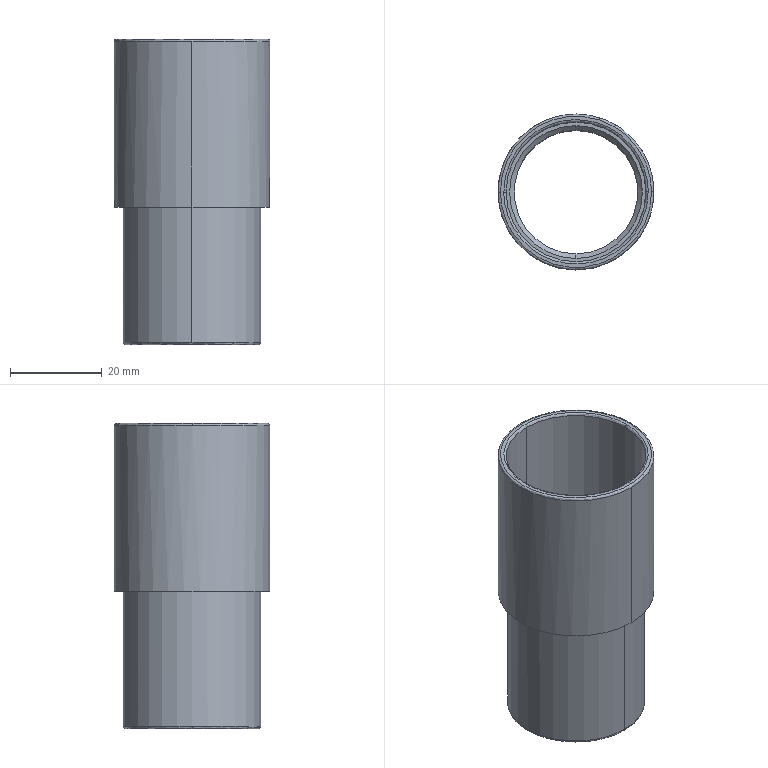Part | SolidWorks | features BaseBody 1 | 1 solid | 20 faces | box 34 x 34 x 66.6 mm | volume 12274 mm3 | cylinder 8 | spline 6 | plane 4 | cone 2 | commonest cylinder face diameters 27 x2 30 x2 30.5 x2 34 x2
STEP:
#1=CARTESIAN_POINT('',(464.037,37.643,-16.634));
#2=VERTEX_POINT('',#1);
#3=CARTESIAN_POINT('',(497.037,37.787,-16.634));
#4=VERTEX_POINT('',#3);
#5=CARTESIAN_POINT('',(464.037,37.643,-16.634));
#6=CARTESIAN_POINT('',(463.893,70.643,-16.634));
#7=CARTESIAN_POINT('',(496.893,70.786,-16.634));
#8=CARTESIAN_POINT('',(497.037,37.787,-16.634));
#9=(BOUNDED_CURVE()B_SPLINE_CURVE(3,(#5,#6,#7,#8),.UNSPECIFIED.,.F.,.T.)B_SPLINE_CURVE_WITH_KNOTS((4,4),(0.,1.),.UNSPECIFIED.)CURVE()GEOMETRIC_REPRESENTATION_ITEM()RATIONAL_B_SPLINE_CURVE((1.,0.3333,0.3333,1.))REPRESENTATION_ITEM(''));
#10=EDGE_CURVE('',#2,#4,#9,.T.);
#11=ORIENTED_EDGE('',*,*,#10,.T.);
#12=CARTESIAN_POINT('',(497.537,37.789,-17.134));
#13=VERTEX_POINT('',#12);
#14=CARTESIAN_POINT('',(497.037,37.787,-17.134));
#15=DIRECTION('',(-0.004352,1.,0.000000003));
#16=DIRECTION('',(1.,0.004352,-0.000000001));
#17=AXIS2_PLACEMENT_3D('',#14,#15,#16);
#18=CIRCLE('',#17,0.5);
#19=EDGE_CURVE('',#4,#13,#18,.T.);
#20=ORIENTED_EDGE('',*,*,#19,.T.);
#21=CARTESIAN_POINT('',(480.537,54.715,-17.134));
#22=VERTEX_POINT('',#21);
#23=CARTESIAN_POINT('',(480.537,37.715,-17.134));
#24=DIRECTION('',(-0.000000001,0.000000003,-1.));
#25=DIRECTION('',(0.,1.,0.000000003));
#26=AXIS2_PLACEMENT_3D('',#23,#24,#25);
#27=CIRCLE('',#26,17.);
#28=EDGE_CURVE('',#22,#13,#27,.T.);
#29=ORIENTED_EDGE('',*,*,#28,.F.);
#30=CARTESIAN_POINT('',(463.537,37.641,-17.134));
#31=VERTEX_POINT('',#30);
#32=CARTESIAN_POINT('',(480.537,37.715,-17.134));
#33=DIRECTION('',(-0.000000001,0.000000003,-1.));
#34=DIRECTION('',(0.,1.,0.000000003));
#35=AXIS2_PLACEMENT_3D('',#32,#33,#34);
#36=CIRCLE('',#35,17.);
#37=EDGE_CURVE('',#31,#22,#36,.T.);
#38=ORIENTED_EDGE('',*,*,#37,.F.);
#39=CARTESIAN_POINT('',(464.037,37.643,-17.134));
#40=DIRECTION('',(0.004352,-1.,-0.000000003));
#41=DIRECTION('',(-1.,-0.004352,0.000000001));
#42=AXIS2_PLACEMENT_3D('',#39,#40,#41);
#43=CIRCLE('',#42,0.5);
#44=EDGE_CURVE('',#2,#31,#43,.T.);
#45=ORIENTED_EDGE('',*,*,#44,.F.);
#46=EDGE_LOOP('',(#11,#20,#29,#38,#45));
#47=FACE_OUTER_BOUND('',#46,.T.);
#48=CARTESIAN_POINT('',(497.037,37.787,-16.634));
#49=CARTESIAN_POINT('',(496.893,70.786,-16.634));
#50=CARTESIAN_POINT('',(463.893,70.643,-16.634));
#51=CARTESIAN_POINT('',(464.037,37.643,-16.634));
#52=CARTESIAN_POINT('',(497.33,37.788,-16.634));
#53=CARTESIAN_POINT('',(497.183,71.373,-16.634));
#54=CARTESIAN_POINT('',(463.598,71.227,-16.634));
#55=CARTESIAN_POINT('',(463.744,37.642,-16.634));
#56=CARTESIAN_POINT('',(497.537,37.789,-16.841));
#57=CARTESIAN_POINT('',(497.389,71.788,-16.841));
#58=CARTESIAN_POINT('',(463.389,71.64,-16.841));
#59=CARTESIAN_POINT('',(463.537,37.641,-16.841));
#60=CARTESIAN_POINT('',(497.537,37.789,-17.134));
#61=CARTESIAN_POINT('',(497.389,71.788,-17.134));
#62=CARTESIAN_POINT('',(463.389,71.64,-17.134));
#63=CARTESIAN_POINT('',(463.537,37.641,-17.134));
#64=(BOUNDED_SURFACE()B_SPLINE_SURFACE(3,3,((#48,#49,#50,#51),(#52,#53,#54,#55),(#56,#57,#58,#59),(#60,#61,#62,#63)),.UNSPECIFIED.,.F.,.F.,.T.)B_SPLINE_SURFACE_WITH_KNOTS((4,4),(4,4),(0.,1.),(0.,1.),.UNSPECIFIED.)GEOMETRIC_REPRESENTATION_ITEM()RATIONAL_B_SPLINE_SURFACE(((1.,0.3333,0.3333,1.),(0.8047,0.2682,0.2682,0.8047),(0.8047,0.2682,0.2682,0.8047),(1.,0.3333,0.3333,1.)))REPRESENTATION_ITEM('')SURFACE());
#65=ADVANCED_FACE('',(#47),#64,.T.);
#66=CARTESIAN_POINT('',(466.037,37.652,-83.234));
#67=VERTEX_POINT('',#66);
#68=CARTESIAN_POINT('',(495.037,37.778,-83.234));
#69=VERTEX_POINT('',#68);
#70=CARTESIAN_POINT('',(466.037,37.652,-83.234));
#71=CARTESIAN_POINT('',(466.163,8.652,-83.234));
#72=CARTESIAN_POINT('',(495.163,8.778,-83.234));
#73=CARTESIAN_POINT('',(495.037,37.778,-83.234));
#74=(BOUNDED_CURVE()B_SPLINE_CURVE(3,(#70,#71,#72,#73),.UNSPECIFIED.,.F.,.T.)B_SPLINE_CURVE_WITH_KNOTS((4,4),(0.,1.),.UNSPECIFIED.)CURVE()GEOMETRIC_REPRESENTATION_ITEM()RATIONAL_B_SPLINE_CURVE((1.,0.3333,0.3333,1.))REPRESENTATION_ITEM(''));
#75=EDGE_CURVE('',#67,#69,#74,.T.);
#76=ORIENTED_EDGE('',*,*,#75,.T.);
#77=CARTESIAN_POINT('',(495.537,37.78,-82.734));
#78=VERTEX_POINT('',#77);
#79=CARTESIAN_POINT('',(495.037,37.778,-82.734));
#80=DIRECTION('',(0.004352,-1.,-0.000000003));
#81=DIRECTION('',(1.,0.004352,-0.000000001));
#82=AXIS2_PLACEMENT_3D('',#79,#80,#81);
#83=CIRCLE('',#82,0.5);
#84=EDGE_CURVE('',#69,#78,#83,.T.);
#85=ORIENTED_EDGE('',*,*,#84,.T.);
#86=CARTESIAN_POINT('',(480.537,22.715,-82.734));
#87=VERTEX_POINT('',#86);
#88=CARTESIAN_POINT('',(480.537,37.715,-82.734));
#89=DIRECTION('',(0.000000001,-0.000000003,1.));
#90=DIRECTION('',(0.,-1.,-0.000000003));
#91=AXIS2_PLACEMENT_3D('',#88,#89,#90);
#92=CIRCLE('',#91,15.);
#93=EDGE_CURVE('',#87,#78,#92,.T.);
#94=ORIENTED_EDGE('',*,*,#93,.F.);
#95=CARTESIAN_POINT('',(465.537,37.649,-82.734));
#96=VERTEX_POINT('',#95);
#97=CARTESIAN_POINT('',(480.537,37.715,-82.734));
#98=DIRECTION('',(0.000000001,-0.000000003,1.));
#99=DIRECTION('',(0.,-1.,-0.000000003));
#100=AXIS2_PLACEMENT_3D('',#97,#98,#99);
#101=CIRCLE('',#100,15.);
#102=EDGE_CURVE('',#96,#87,#101,.T.);
#103=ORIENTED_EDGE('',*,*,#102,.F.);
#104=CARTESIAN_POINT('',(466.037,37.652,-82.734));
#105=DIRECTION('',(-0.004352,1.,0.000000003));
#106=DIRECTION('',(-1.,-0.004352,0.000000001));
#107=AXIS2_PLACEMENT_3D('',#104,#105,#106);
#108=CIRCLE('',#107,0.5);
#109=EDGE_CURVE('',#67,#96,#108,.T.);
#110=ORIENTED_EDGE('',*,*,#109,.F.);
#111=EDGE_LOOP('',(#76,#85,#94,#103,#110));
#112=FACE_OUTER_BOUND('',#111,.T.);
#113=CARTESIAN_POINT('',(495.037,37.778,-83.234));
#114=CARTESIAN_POINT('',(495.163,8.778,-83.234));
#115=CARTESIAN_POINT('',(466.163,8.652,-83.234));
#116=CARTESIAN_POINT('',(466.037,37.652,-83.234));
#117=CARTESIAN_POINT('',(495.33,37.779,-83.234));
#118=CARTESIAN_POINT('',(495.458,8.194,-83.234));
#119=CARTESIAN_POINT('',(465.873,8.065,-83.234));
#120=CARTESIAN_POINT('',(465.744,37.65,-83.234));
#121=CARTESIAN_POINT('',(495.537,37.78,-83.027));
#122=CARTESIAN_POINT('',(495.667,7.78,-83.027));
#123=CARTESIAN_POINT('',(465.668,7.65,-83.027));
#124=CARTESIAN_POINT('',(465.537,37.649,-83.027));
#125=CARTESIAN_POINT('',(495.537,37.78,-82.734));
#126=CARTESIAN_POINT('',(495.667,7.78,-82.734));
#127=CARTESIAN_POINT('',(465.668,7.65,-82.734));
#128=CARTESIAN_POINT('',(465.537,37.649,-82.734));
#129=(BOUNDED_SURFACE()B_SPLINE_SURFACE(3,3,((#113,#114,#115,#116),(#117,#118,#119,#120),(#121,#122,#123,#124),(#125,#126,#127,#128)),.UNSPECIFIED.,.F.,.F.,.T.)B_SPLINE_SURFACE_WITH_KNOTS((4,4),(4,4),(0.,1.),(0.,1.),.UNSPECIFIED.)GEOMETRIC_REPRESENTATION_ITEM()RATIONAL_B_SPLINE_SURFACE(((1.,0.3333,0.3333,1.),(0.8047,0.2682,0.2682,0.8047),(0.8047,0.2682,0.2682,0.8047),(1.,0.3333,0.3333,1.)))REPRESENTATION_ITEM('')SURFACE());
#130=ADVANCED_FACE('',(#112),#129,.T.);
#131=CARTESIAN_POINT('',(480.537,52.965,-17.134));
#132=VERTEX_POINT('',#131);
#133=CARTESIAN_POINT('',(495.787,37.781,-17.134));
#134=VERTEX_POINT('',#133);
#135=CARTESIAN_POINT('',(480.537,37.715,-17.134));
#136=DIRECTION('',(-0.000000001,0.000000003,-1.));
#137=DIRECTION('',(-1.,-0.004352,0.000000001));
#138=AXIS2_PLACEMENT_3D('',#135,#136,#137);
#139=CIRCLE('',#138,15.25);
#140=EDGE_CURVE('',#132,#134,#139,.T.);
#141=ORIENTED_EDGE('',*,*,#140,.T.);
#142=CARTESIAN_POINT('',(496.287,37.783,-16.634));
#143=VERTEX_POINT('',#142);
#144=CARTESIAN_POINT('',(496.287,37.783,-17.134));
#145=DIRECTION('',(-0.004352,1.,0.000000003));
#146=DIRECTION('',(1.,0.004352,-0.000000001));
#147=AXIS2_PLACEMENT_3D('',#144,#145,#146);
#148=CIRCLE('',#147,0.5);
#149=EDGE_CURVE('',#134,#143,#148,.T.);
#150=ORIENTED_EDGE('',*,*,#149,.T.);
#151=CARTESIAN_POINT('',(464.787,37.646,-16.634));
#152=VERTEX_POINT('',#151);
#153=CARTESIAN_POINT('',(464.787,37.646,-16.634));
#154=CARTESIAN_POINT('',(464.785,38.128,-16.634));
#155=CARTESIAN_POINT('',(464.815,38.847,-16.634));
#156=CARTESIAN_POINT('',(464.907,39.682,-16.634));
#157=CARTESIAN_POINT('',(464.967,40.098,-16.634));
#158=CARTESIAN_POINT('',(465.001,40.306,-16.634));
#159=CARTESIAN_POINT('',(465.017,40.395,-16.634));
#160=CARTESIAN_POINT('',(465.027,40.454,-16.634));
#161=CARTESIAN_POINT('',(465.032,40.482,-16.634));
#162=CARTESIAN_POINT('',(465.128,41.016,-16.634));
#163=CARTESIAN_POINT('',(465.3,41.759,-16.634));
#164=CARTESIAN_POINT('',(465.563,42.61,-16.634));
#165=CARTESIAN_POINT('',(465.71,43.031,-16.634));
#166=CARTESIAN_POINT('',(465.788,43.24,-16.634));
#167=CARTESIAN_POINT('',(465.822,43.329,-16.634));
#168=CARTESIAN_POINT('',(465.844,43.389,-16.634));
#169=CARTESIAN_POINT('',(465.855,43.417,-16.634));
#170=CARTESIAN_POINT('',(466.061,43.944,-16.634));
#171=CARTESIAN_POINT('',(466.388,44.669,-16.634));
#172=CARTESIAN_POINT('',(466.831,45.483,-16.634));
#173=CARTESIAN_POINT('',(467.069,45.882,-16.634));
#174=CARTESIAN_POINT('',(467.174,46.051,-16.634));
#175=CARTESIAN_POINT('',(467.245,46.164,-16.634));
#176=CARTESIAN_POINT('',(467.28,46.219,-16.634));
#177=CARTESIAN_POINT('',(467.908,47.188,-16.634));
#178=CARTESIAN_POINT('',(468.586,48.031,-16.634));
#179=CARTESIAN_POINT('',(469.734,49.189,-16.634));
#180=CARTESIAN_POINT('',(470.335,49.736,-16.634));
#181=CARTESIAN_POINT('',(471.082,50.317,-16.634));
#182=CARTESIAN_POINT('',(471.468,50.593,-16.634));
#183=CARTESIAN_POINT('',(471.635,50.708,-16.634));
#184=CARTESIAN_POINT('',(471.748,50.785,-16.634));
#185=CARTESIAN_POINT('',(471.806,50.823,-16.634));
#186=CARTESIAN_POINT('',(472.305,51.153,-16.634));
#187=CARTESIAN_POINT('',(472.99,51.557,-16.634));
#188=CARTESIAN_POINT('',(473.822,51.966,-16.634));
#189=CARTESIAN_POINT('',(474.246,52.155,-16.634));
#190=CARTESIAN_POINT('',(474.46,52.246,-16.634));
#191=CARTESIAN_POINT('',(474.552,52.284,-16.634));
#192=CARTESIAN_POINT('',(474.614,52.309,-16.634));
#193=CARTESIAN_POINT('',(474.646,52.322,-16.634));
#194=CARTESIAN_POINT('',(475.15,52.524,-16.634));
#195=CARTESIAN_POINT('',(475.871,52.773,-16.634));
#196=CARTESIAN_POINT('',(476.731,53.002,-16.634));
#197=CARTESIAN_POINT('',(477.166,53.101,-16.634));
#198=CARTESIAN_POINT('',(477.384,53.146,-16.634));
#199=CARTESIAN_POINT('',(477.478,53.165,-16.634));
#200=CARTESIAN_POINT('',(477.541,53.177,-16.634));
#201=CARTESIAN_POINT('',(477.574,53.184,-16.634));
#202=CARTESIAN_POINT('',(478.55,53.369,-16.634));
#203=CARTESIAN_POINT('',(479.505,53.46,-16.634));
#204=CARTESIAN_POINT('',(480.95,53.467,-16.634));
#205=CARTESIAN_POINT('',(481.669,53.437,-16.634));
#206=CARTESIAN_POINT('',(482.504,53.345,-16.634));
#207=CARTESIAN_POINT('',(482.92,53.284,-16.634));
#208=CARTESIAN_POINT('',(483.128,53.25,-16.634));
#209=CARTESIAN_POINT('',(483.217,53.235,-16.634));
#210=CARTESIAN_POINT('',(483.276,53.225,-16.634));
#211=CARTESIAN_POINT('',(483.304,53.22,-16.634));
#212=CARTESIAN_POINT('',(483.838,53.123,-16.634));
#213=CARTESIAN_POINT('',(484.582,52.952,-16.634));
#214=CARTESIAN_POINT('',(485.432,52.689,-16.634));
#215=CARTESIAN_POINT('',(485.853,52.542,-16.634));
#216=CARTESIAN_POINT('',(486.062,52.464,-16.634));
#217=CARTESIAN_POINT('',(486.151,52.43,-16.634));
#218=CARTESIAN_POINT('',(486.211,52.407,-16.634));
#219=CARTESIAN_POINT('',(486.24,52.396,-16.634));
#220=CARTESIAN_POINT('',(486.766,52.19,-16.634));
#221=CARTESIAN_POINT('',(487.491,51.864,-16.634));
#222=CARTESIAN_POINT('',(488.305,51.42,-16.634));
#223=CARTESIAN_POINT('',(488.704,51.183,-16.634));
#224=CARTESIAN_POINT('',(488.874,51.078,-16.634));
#225=CARTESIAN_POINT('',(488.986,51.007,-16.634));
#226=CARTESIAN_POINT('',(489.041,50.972,-16.634));
#227=CARTESIAN_POINT('',(490.01,50.344,-16.634));
#228=CARTESIAN_POINT('',(490.853,49.665,-16.634));
#229=CARTESIAN_POINT('',(492.011,48.517,-16.634));
#230=CARTESIAN_POINT('',(492.558,47.917,-16.634));
#231=CARTESIAN_POINT('',(493.139,47.169,-16.634));
#232=CARTESIAN_POINT('',(493.415,46.784,-16.634));
#233=CARTESIAN_POINT('',(493.53,46.616,-16.634));
#234=CARTESIAN_POINT('',(493.607,46.504,-16.634));
#235=CARTESIAN_POINT('',(493.645,46.446,-16.634));
#236=CARTESIAN_POINT('',(493.975,45.946,-16.634));
#237=CARTESIAN_POINT('',(494.379,45.262,-16.634));
#238=CARTESIAN_POINT('',(494.788,44.43,-16.634));
#239=CARTESIAN_POINT('',(494.977,44.006,-16.634));
#240=CARTESIAN_POINT('',(495.068,43.791,-16.634));
#241=CARTESIAN_POINT('',(495.106,43.699,-16.634));
#242=CARTESIAN_POINT('',(495.131,43.638,-16.634));
#243=CARTESIAN_POINT('',(495.144,43.606,-16.634));
#244=CARTESIAN_POINT('',(495.346,43.102,-16.634));
#245=CARTESIAN_POINT('',(495.595,42.381,-16.634));
#246=CARTESIAN_POINT('',(495.824,41.52,-16.634));
#247=CARTESIAN_POINT('',(495.923,41.086,-16.634));
#248=CARTESIAN_POINT('',(495.968,40.867,-16.634));
#249=CARTESIAN_POINT('',(495.987,40.773,-16.634));
#250=CARTESIAN_POINT('',(495.999,40.711,-16.634));
#251=CARTESIAN_POINT('',(496.006,40.678,-16.634));
#252=CARTESIAN_POINT('',(496.191,39.702,-16.634));
#253=CARTESIAN_POINT('',(496.283,38.747,-16.634));
#254=CARTESIAN_POINT('',(496.287,37.783,-16.634));
#255=B_SPLINE_CURVE_WITH_KNOTS('',3,(#153,#154,#155,#156,#157,#158,#159,#160,#161,#162,#163,#164,#165,#166,#167,#168,#169,#170,#171,#172,#173,#174,#175,#176,#177,#178,#179,#180,#181,#182,#183,#184,#185,#186,#187,#188,#189,#190,#191,#192,#193,#194,#195,#196,#197,#198,#199,#200,#201,#202,#203,#204,#205,#206,#207,#208,#209,#210,#211,#212,#213,#214,#215,#216,#217,#218,#219,#220,#221,#222,#223,#224,#225,#226,#227,#228,#229,#230,#231,#232,#233,#234,#235,#236,#237,#238,#239,#240,#241,#242,#243,#244,#245,#246,#247,#248,#249,#250,#251,#252,#253,#254),.UNSPECIFIED.,.F.,.F.,(4,1,1,1,1,2,2,1,1,1,1,2,2,1,1,1,2,2,2,1,1,1,2,2,1,1,1,1,2,2,1,1,1,1,2,2,2,1,1,1,1,2,2,1,1,1,1,2,2,1,1,1,2,2,2,1,1,1,2,2,1,1,1,1,2,2,1,1,1,1,2,2,4),(0.,0.03125,0.04687,0.05469,0.05859,0.06055,0.0625,0.09375,0.1094,0.1172,0.1211,0.123,0.125,0.1562,0.1719,0.1797,0.1836,0.1875,0.25,0.2812,0.2969,0.3047,0.3086,0.3125,0.3437,0.3594,0.3672,0.3711,0.373,0.375,0.4062,0.4219,0.4297,0.4336,0.4355,0.4375,0.5,0.5312,0.5469,0.5547,0.5586,0.5605,0.5625,0.5937,0.6094,0.6172,0.6211,0.623,0.625,0.6562,0.6719,0.6797,0.6836,0.6875,0.75,0.7812,0.7969,0.8047,0.8086,0.8125,0.8437,0.8594,0.8672,0.8711,0.873,0.875,0.9062,0.9219,0.9297,0.9336,0.9355,0.9375,1.),.UNSPECIFIED.);
#256=EDGE_CURVE('',#152,#143,#255,.T.);
#257=ORIENTED_EDGE('',*,*,#256,.F.);
#258=CARTESIAN_POINT('',(465.287,37.648,-17.134));
#259=VERTEX_POINT('',#258);
#260=CARTESIAN_POINT('',(464.787,37.646,-17.134));
#261=DIRECTION('',(0.004352,-1.,-0.000000003));
#262=DIRECTION('',(-1.,-0.004352,0.000000001));
#263=AXIS2_PLACEMENT_3D('',#260,#261,#262);
#264=CIRCLE('',#263,0.5);
#265=EDGE_CURVE('',#259,#152,#264,.T.);
#266=ORIENTED_EDGE('',*,*,#265,.F.);
#267=CARTESIAN_POINT('',(480.537,37.715,-17.134));
#268=DIRECTION('',(-0.000000001,0.000000003,-1.));
#269=DIRECTION('',(-1.,-0.004352,0.000000001));
#270=AXIS2_PLACEMENT_3D('',#267,#268,#269);
#271=CIRCLE('',#270,15.25);
#272=EDGE_CURVE('',#259,#132,#271,.T.);
#273=ORIENTED_EDGE('',*,*,#272,.T.);
#274=EDGE_LOOP('',(#141,#150,#257,#266,#273));
#275=FACE_OUTER_BOUND('',#274,.T.);
#276=CARTESIAN_POINT('',(495.787,37.781,-17.134));
#277=CARTESIAN_POINT('',(495.654,68.281,-17.134));
#278=CARTESIAN_POINT('',(465.154,68.148,-17.134));
#279=CARTESIAN_POINT('',(465.287,37.648,-17.134));
#280=CARTESIAN_POINT('',(495.787,37.781,-16.841));
#281=CARTESIAN_POINT('',(495.654,68.281,-16.841));
#282=CARTESIAN_POINT('',(465.154,68.148,-16.841));
#283=CARTESIAN_POINT('',(465.287,37.648,-16.841));
#284=CARTESIAN_POINT('',(495.994,37.782,-16.634));
#285=CARTESIAN_POINT('',(495.859,68.696,-16.634));
#286=CARTESIAN_POINT('',(464.945,68.561,-16.634));
#287=CARTESIAN_POINT('',(465.08,37.647,-16.634));
#288=CARTESIAN_POINT('',(496.287,37.783,-16.634));
#289=CARTESIAN_POINT('',(496.15,69.283,-16.634));
#290=CARTESIAN_POINT('',(464.65,69.146,-16.634));
#291=CARTESIAN_POINT('',(464.787,37.646,-16.634));
#292=(BOUNDED_SURFACE()B_SPLINE_SURFACE(3,3,((#276,#277,#278,#279),(#280,#281,#282,#283),(#284,#285,#286,#287),(#288,#289,#290,#291)),.UNSPECIFIED.,.F.,.F.,.T.)B_SPLINE_SURFACE_WITH_KNOTS((4,4),(4,4),(0.,1.),(0.,1.),.UNSPECIFIED.)GEOMETRIC_REPRESENTATION_ITEM()RATIONAL_B_SPLINE_SURFACE(((1.,0.3333,0.3333,1.),(0.8047,0.2682,0.2682,0.8047),(0.8047,0.2682,0.2682,0.8047),(1.,0.3333,0.3333,1.)))REPRESENTATION_ITEM('')SURFACE());
#293=ADVANCED_FACE('',(#275),#292,.T.);
#294=ORIENTED_EDGE('',*,*,#28,.T.);
#295=CARTESIAN_POINT('',(480.537,20.715,-17.134));
#296=VERTEX_POINT('',#295);
#297=CARTESIAN_POINT('',(480.537,37.715,-17.134));
#298=DIRECTION('',(-0.000000001,0.000000003,-1.));
#299=DIRECTION('',(0.,1.,0.000000003));
#300=AXIS2_PLACEMENT_3D('',#297,#298,#299);
#301=CIRCLE('',#300,17.);
#302=EDGE_CURVE('',#13,#296,#301,.T.);
#303=ORIENTED_EDGE('',*,*,#302,.T.);
#304=CARTESIAN_POINT('',(480.537,20.715,-53.23));
#305=VERTEX_POINT('',#304);
#306=CARTESIAN_POINT('',(480.537,20.715,-53.23));
#307=DIRECTION('',(-0.000000001,0.000000003,-1.));
#308=VECTOR('',#307,1000.);
#309=LINE('',#306,#308);
#310=EDGE_CURVE('',#296,#305,#309,.T.);
#311=ORIENTED_EDGE('',*,*,#310,.T.);
#312=CARTESIAN_POINT('',(480.537,54.715,-53.23));
#313=VERTEX_POINT('',#312);
#314=CARTESIAN_POINT('',(480.537,37.715,-53.23));
#315=DIRECTION('',(0.000000001,-0.000000003,1.));
#316=DIRECTION('',(0.,1.,0.000000003));
#317=AXIS2_PLACEMENT_3D('',#314,#315,#316);
#318=CIRCLE('',#317,17.);
#319=EDGE_CURVE('',#305,#313,#318,.T.);
#320=ORIENTED_EDGE('',*,*,#319,.T.);
#321=CARTESIAN_POINT('',(480.537,54.715,-53.23));
#322=DIRECTION('',(-0.000000001,0.000000003,-1.));
#323=VECTOR('',#322,1000.);
#324=LINE('',#321,#323);
#325=EDGE_CURVE('',#22,#313,#324,.T.);
#326=ORIENTED_EDGE('',*,*,#325,.F.);
#327=EDGE_LOOP('',(#294,#303,#311,#320,#326));
#328=FACE_OUTER_BOUND('',#327,.T.);
#329=CARTESIAN_POINT('',(480.537,37.715,-53.23));
#330=DIRECTION('',(-0.000000001,0.000000003,-1.));
#331=DIRECTION('',(0.,1.,0.000000003));
#332=AXIS2_PLACEMENT_3D('',#329,#330,#331);
#333=CYLINDRICAL_SURFACE('',#332,17.);
#334=ADVANCED_FACE('',(#328),#333,.T.);
#335=ORIENTED_EDGE('',*,*,#93,.T.);
#336=CARTESIAN_POINT('',(480.537,52.715,-82.734));
#337=VERTEX_POINT('',#336);
#338=CARTESIAN_POINT('',(480.537,37.715,-82.734));
#339=DIRECTION('',(0.000000001,-0.000000003,1.));
#340=DIRECTION('',(0.,-1.,-0.000000003));
#341=AXIS2_PLACEMENT_3D('',#338,#339,#340);
#342=CIRCLE('',#341,15.);
#343=EDGE_CURVE('',#78,#337,#342,.T.);
#344=ORIENTED_EDGE('',*,*,#343,.T.);
#345=CARTESIAN_POINT('',(480.537,52.715,-53.23));
#346=VERTEX_POINT('',#345);
#347=CARTESIAN_POINT('',(480.537,52.715,-53.23));
#348=DIRECTION('',(0.000000001,-0.000000003,1.));
#349=VECTOR('',#348,1000.);
#350=LINE('',#347,#349);
#351=EDGE_CURVE('',#337,#346,#350,.T.);
#352=ORIENTED_EDGE('',*,*,#351,.T.);
#353=CARTESIAN_POINT('',(480.537,22.715,-53.23));
#354=VERTEX_POINT('',#353);
#355=CARTESIAN_POINT('',(480.537,37.715,-53.23));
#356=DIRECTION('',(-0.000000001,0.000000003,-1.));
#357=DIRECTION('',(0.,-1.,-0.000000003));
#358=AXIS2_PLACEMENT_3D('',#355,#356,#357);
#359=CIRCLE('',#358,15.);
#360=EDGE_CURVE('',#346,#354,#359,.T.);
#361=ORIENTED_EDGE('',*,*,#360,.T.);
#362=CARTESIAN_POINT('',(480.537,22.715,-53.23));
#363=DIRECTION('',(0.000000001,-0.000000003,1.));
#364=VECTOR('',#363,1000.);
#365=LINE('',#362,#364);
#366=EDGE_CURVE('',#87,#354,#365,.T.);
#367=ORIENTED_EDGE('',*,*,#366,.F.);
#368=EDGE_LOOP('',(#335,#344,#352,#361,#367));
#369=FACE_OUTER_BOUND('',#368,.T.);
#370=CARTESIAN_POINT('',(480.537,37.715,-53.23));
#371=DIRECTION('',(0.000000001,-0.000000003,1.));
#372=DIRECTION('',(0.,-1.,-0.000000003));
#373=AXIS2_PLACEMENT_3D('',#370,#371,#372);
#374=CYLINDRICAL_SURFACE('',#373,15.);
#375=ADVANCED_FACE('',(#369),#374,.T.);
#376=CARTESIAN_POINT('',(480.537,52.965,-41.634));
#377=VERTEX_POINT('',#376);
#378=CARTESIAN_POINT('',(480.537,22.465,-41.634));
#379=VERTEX_POINT('',#378);
#380=CARTESIAN_POINT('',(480.537,37.715,-41.634));
#381=DIRECTION('',(0.000000001,-0.000000003,1.));
#382=DIRECTION('',(0.,-1.,-0.000000003));
#383=AXIS2_PLACEMENT_3D('',#380,#381,#382);
#384=CIRCLE('',#383,15.25);
#385=EDGE_CURVE('',#377,#379,#384,.T.);
#386=ORIENTED_EDGE('',*,*,#385,.F.);
#387=CARTESIAN_POINT('',(480.537,52.965,-16.634));
#388=DIRECTION('',(0.000000001,-0.000000003,1.));
#389=VECTOR('',#388,1000.);
#390=LINE('',#387,#389);
#391=EDGE_CURVE('',#377,#132,#390,.T.);
#392=ORIENTED_EDGE('',*,*,#391,.T.);
#393=ORIENTED_EDGE('',*,*,#272,.F.);
#394=CARTESIAN_POINT('',(480.537,22.465,-17.134));
#395=VERTEX_POINT('',#394);
#396=CARTESIAN_POINT('',(480.537,37.715,-17.134));
#397=DIRECTION('',(-0.000000001,0.000000003,-1.));
#398=DIRECTION('',(-1.,-0.004352,0.000000001));
#399=AXIS2_PLACEMENT_3D('',#396,#397,#398);
#400=CIRCLE('',#399,15.25);
#401=EDGE_CURVE('',#395,#259,#400,.T.);
#402=ORIENTED_EDGE('',*,*,#401,.F.);
#403=CARTESIAN_POINT('',(480.537,22.465,-16.634));
#404=DIRECTION('',(0.000000001,-0.000000003,1.));
#405=VECTOR('',#404,1000.);
#406=LINE('',#403,#405);
#407=EDGE_CURVE('',#379,#395,#406,.T.);
#408=ORIENTED_EDGE('',*,*,#407,.F.);
#409=EDGE_LOOP('',(#386,#392,#393,#402,#408));
#410=FACE_OUTER_BOUND('',#409,.T.);
#411=CARTESIAN_POINT('',(480.537,37.715,-16.634));
#412=DIRECTION('',(0.000000001,-0.000000003,1.));
#413=DIRECTION('',(0.,-1.,-0.000000003));
#414=AXIS2_PLACEMENT_3D('',#411,#412,#413);
#415=CYLINDRICAL_SURFACE('',#414,15.25);
#416=ADVANCED_FACE('',(#410),#415,.F.);
#417=CARTESIAN_POINT('',(480.537,51.215,-83.234));
#418=VERTEX_POINT('',#417);
#419=CARTESIAN_POINT('',(480.537,24.215,-83.234));
#420=VERTEX_POINT('',#419);
#421=CARTESIAN_POINT('',(480.537,37.715,-83.234));
#422=DIRECTION('',(0.000000001,-0.000000003,1.));
#423=DIRECTION('',(0.,-1.,-0.000000003));
#424=AXIS2_PLACEMENT_3D('',#421,#422,#423);
#425=CIRCLE('',#424,13.5);
#426=EDGE_CURVE('',#418,#420,#425,.T.);
#427=ORIENTED_EDGE('',*,*,#426,.F.);
#428=CARTESIAN_POINT('',(480.537,51.215,-42.634));
#429=VERTEX_POINT('',#428);
#430=CARTESIAN_POINT('',(480.537,51.215,-16.634));
#431=DIRECTION('',(0.000000001,-0.000000003,1.));
#432=VECTOR('',#431,1000.);
#433=LINE('',#430,#432);
#434=EDGE_CURVE('',#418,#429,#433,.T.);
#435=ORIENTED_EDGE('',*,*,#434,.T.);
#436=CARTESIAN_POINT('',(480.537,24.215,-42.634));
#437=VERTEX_POINT('',#436);
#438=CARTESIAN_POINT('',(480.537,37.715,-42.634));
#439=DIRECTION('',(-0.000000001,0.000000003,-1.));
#440=DIRECTION('',(0.,-1.,-0.000000003));
#441=AXIS2_PLACEMENT_3D('',#438,#439,#440);
#442=CIRCLE('',#441,13.5);
#443=EDGE_CURVE('',#437,#429,#442,.T.);
#444=ORIENTED_EDGE('',*,*,#443,.F.);
#445=CARTESIAN_POINT('',(480.537,24.215,-16.634));
#446=DIRECTION('',(0.000000001,-0.000000003,1.));
#447=VECTOR('',#446,1000.);
#448=LINE('',#445,#447);
#449=EDGE_CURVE('',#420,#437,#448,.T.);
#450=ORIENTED_EDGE('',*,*,#449,.F.);
#451=EDGE_LOOP('',(#427,#435,#444,#450));
#452=FACE_OUTER_BOUND('',#451,.T.);
#453=CARTESIAN_POINT('',(480.537,37.715,-16.634));
#454=DIRECTION('',(0.000000001,-0.000000003,1.));
#455=DIRECTION('',(0.,-1.,-0.000000003));
#456=AXIS2_PLACEMENT_3D('',#453,#454,#455);
#457=CYLINDRICAL_SURFACE('',#456,13.5);
#458=ADVANCED_FACE('',(#452),#457,.F.);
#459=ORIENTED_EDGE('',*,*,#443,.T.);
#460=CARTESIAN_POINT('',(480.537,52.215,-41.634));
#461=VERTEX_POINT('',#460);
#462=CARTESIAN_POINT('',(480.537,52.215,-41.634));
#463=DIRECTION('',(0.000000001,0.7071,0.7071));
#464=VECTOR('',#463,1000.);
#465=LINE('',#462,#464);
#466=EDGE_CURVE('',#429,#461,#465,.T.);
#467=ORIENTED_EDGE('',*,*,#466,.T.);
#468=CARTESIAN_POINT('',(480.537,23.215,-41.634));
#469=VERTEX_POINT('',#468);
#470=CARTESIAN_POINT('',(480.537,37.715,-41.634));
#471=DIRECTION('',(0.000000001,-0.000000003,1.));
#472=DIRECTION('',(0.,-1.,-0.000000003));
#473=AXIS2_PLACEMENT_3D('',#470,#471,#472);
#474=CIRCLE('',#473,14.5);
#475=EDGE_CURVE('',#461,#469,#474,.T.);
#476=ORIENTED_EDGE('',*,*,#475,.T.);
#477=CARTESIAN_POINT('',(480.537,23.215,-41.634));
#478=DIRECTION('',(0.000000001,-0.7071,0.7071));
#479=VECTOR('',#478,1000.);
#480=LINE('',#477,#479);
#481=EDGE_CURVE('',#437,#469,#480,.T.);
#482=ORIENTED_EDGE('',*,*,#481,.F.);
#483=EDGE_LOOP('',(#459,#467,#476,#482));
#484=FACE_OUTER_BOUND('',#483,.T.);
#485=CARTESIAN_POINT('',(480.537,37.715,-41.634));
#486=DIRECTION('',(0.000000001,-0.000000003,1.));
#487=DIRECTION('',(0.,-1.,-0.000000003));
#488=AXIS2_PLACEMENT_3D('',#485,#486,#487);
#489=CONICAL_SURFACE('',#488,14.5,0.7854);
#490=ADVANCED_FACE('',(#484),#489,.F.);
#491=ORIENTED_EDGE('',*,*,#310,.F.);
#492=CARTESIAN_POINT('',(480.537,37.715,-17.134));
#493=DIRECTION('',(-0.000000001,0.000000003,-1.));
#494=DIRECTION('',(0.,1.,0.000000003));
#495=AXIS2_PLACEMENT_3D('',#492,#493,#494);
#496=CIRCLE('',#495,17.);
#497=EDGE_CURVE('',#296,#31,#496,.T.);
#498=ORIENTED_EDGE('',*,*,#497,.T.);
#499=ORIENTED_EDGE('',*,*,#37,.T.);
#500=ORIENTED_EDGE('',*,*,#325,.T.);
#501=CARTESIAN_POINT('',(480.537,37.715,-53.23));
#502=DIRECTION('',(0.000000001,-0.000000003,1.));
#503=DIRECTION('',(0.,1.,0.000000003));
#504=AXIS2_PLACEMENT_3D('',#501,#502,#503);
#505=CIRCLE('',#504,17.);
#506=EDGE_CURVE('',#313,#305,#505,.T.);
#507=ORIENTED_EDGE('',*,*,#506,.T.);
#508=EDGE_LOOP('',(#491,#498,#499,#500,#507));
#509=FACE_OUTER_BOUND('',#508,.T.);
#510=CARTESIAN_POINT('',(480.537,37.715,-53.23));
#511=DIRECTION('',(-0.000000001,0.000000003,-1.));
#512=DIRECTION('',(0.,1.,0.000000003));
#513=AXIS2_PLACEMENT_3D('',#510,#511,#512);
#514=CYLINDRICAL_SURFACE('',#513,17.);
#515=ADVANCED_FACE('',(#509),#514,.T.);
#516=ORIENTED_EDGE('',*,*,#506,.F.);
#517=ORIENTED_EDGE('',*,*,#319,.F.);
#518=EDGE_LOOP('',(#516,#517));
#519=FACE_OUTER_BOUND('',#518,.T.);
#520=CARTESIAN_POINT('',(480.537,37.715,-53.23));
#521=DIRECTION('',(-0.000000001,0.000000003,-1.));
#522=DIRECTION('',(0.,-1.,-0.000000003));
#523=AXIS2_PLACEMENT_3D('',#520,#521,#522);
#524=CIRCLE('',#523,15.);
#525=EDGE_CURVE('',#354,#346,#524,.T.);
#526=ORIENTED_EDGE('',*,*,#525,.F.);
#527=ORIENTED_EDGE('',*,*,#360,.F.);
#528=EDGE_LOOP('',(#526,#527));
#529=FACE_BOUND('',#528,.T.);
#530=CARTESIAN_POINT('',(480.537,37.715,-53.23));
#531=DIRECTION('',(0.000000001,-0.000000003,1.));
#532=DIRECTION('',(0.,-1.,-0.000000003));
#533=AXIS2_PLACEMENT_3D('',#530,#531,#532);
#534=PLANE('',#533);
#535=ADVANCED_FACE('',(#519,#529),#534,.F.);
#536=ORIENTED_EDGE('',*,*,#19,.F.);
#537=CARTESIAN_POINT('',(497.037,37.787,-16.634));
#538=CARTESIAN_POINT('',(497.18,4.787,-16.634));
#539=CARTESIAN_POINT('',(464.181,4.643,-16.634));
#540=CARTESIAN_POINT('',(464.037,37.643,-16.634));
#541=(BOUNDED_CURVE()B_SPLINE_CURVE(3,(#537,#538,#539,#540),.UNSPECIFIED.,.F.,.F.)B_SPLINE_CURVE_WITH_KNOTS((4,4),(0.,1.),.UNSPECIFIED.)CURVE()GEOMETRIC_REPRESENTATION_ITEM()RATIONAL_B_SPLINE_CURVE((1.,0.3333,0.3333,1.))REPRESENTATION_ITEM(''));
#542=EDGE_CURVE('',#4,#2,#541,.T.);
#543=ORIENTED_EDGE('',*,*,#542,.T.);
#544=ORIENTED_EDGE('',*,*,#44,.T.);
#545=ORIENTED_EDGE('',*,*,#497,.F.);
#546=ORIENTED_EDGE('',*,*,#302,.F.);
#547=EDGE_LOOP('',(#536,#543,#544,#545,#546));
#548=FACE_OUTER_BOUND('',#547,.T.);
#549=CARTESIAN_POINT('',(464.037,37.643,-16.634));
#550=CARTESIAN_POINT('',(464.181,4.643,-16.634));
#551=CARTESIAN_POINT('',(497.18,4.787,-16.634));
#552=CARTESIAN_POINT('',(497.037,37.787,-16.634));
#553=CARTESIAN_POINT('',(463.744,37.642,-16.634));
#554=CARTESIAN_POINT('',(463.89,4.056,-16.634));
#555=CARTESIAN_POINT('',(497.476,4.202,-16.634));
#556=CARTESIAN_POINT('',(497.33,37.788,-16.634));
#557=CARTESIAN_POINT('',(463.537,37.641,-16.841));
#558=CARTESIAN_POINT('',(463.685,3.641,-16.841));
#559=CARTESIAN_POINT('',(497.685,3.789,-16.841));
#560=CARTESIAN_POINT('',(497.537,37.789,-16.841));
#561=CARTESIAN_POINT('',(463.537,37.641,-17.134));
#562=CARTESIAN_POINT('',(463.685,3.641,-17.134));
#563=CARTESIAN_POINT('',(497.685,3.789,-17.134));
#564=CARTESIAN_POINT('',(497.537,37.789,-17.134));
#565=(BOUNDED_SURFACE()B_SPLINE_SURFACE(3,3,((#549,#550,#551,#552),(#553,#554,#555,#556),(#557,#558,#559,#560),(#561,#562,#563,#564)),.UNSPECIFIED.,.F.,.F.,.F.)B_SPLINE_SURFACE_WITH_KNOTS((4,4),(4,4),(0.,1.),(0.,1.),.UNSPECIFIED.)GEOMETRIC_REPRESENTATION_ITEM()RATIONAL_B_SPLINE_SURFACE(((1.,0.3333,0.3333,1.),(0.8047,0.2682,0.2682,0.8047),(0.8047,0.2682,0.2682,0.8047),(1.,0.3333,0.3333,1.)))REPRESENTATION_ITEM('')SURFACE());
#566=ADVANCED_FACE('',(#548),#565,.T.);
#567=ORIENTED_EDGE('',*,*,#351,.F.);
#568=CARTESIAN_POINT('',(480.537,37.715,-82.734));
#569=DIRECTION('',(0.000000001,-0.000000003,1.));
#570=DIRECTION('',(0.,-1.,-0.000000003));
#571=AXIS2_PLACEMENT_3D('',#568,#569,#570);
#572=CIRCLE('',#571,15.);
#573=EDGE_CURVE('',#337,#96,#572,.T.);
#574=ORIENTED_EDGE('',*,*,#573,.T.);
#575=ORIENTED_EDGE('',*,*,#102,.T.);
#576=ORIENTED_EDGE('',*,*,#366,.T.);
#577=ORIENTED_EDGE('',*,*,#525,.T.);
#578=EDGE_LOOP('',(#567,#574,#575,#576,#577));
#579=FACE_OUTER_BOUND('',#578,.T.);
#580=CARTESIAN_POINT('',(480.537,37.715,-53.23));
#581=DIRECTION('',(0.000000001,-0.000000003,1.));
#582=DIRECTION('',(0.,-1.,-0.000000003));
#583=AXIS2_PLACEMENT_3D('',#580,#581,#582);
#584=CYLINDRICAL_SURFACE('',#583,15.);
#585=ADVANCED_FACE('',(#579),#584,.T.);
#586=ORIENTED_EDGE('',*,*,#542,.F.);
#587=ORIENTED_EDGE('',*,*,#10,.F.);
#588=EDGE_LOOP('',(#586,#587));
#589=FACE_OUTER_BOUND('',#588,.T.);
#590=ORIENTED_EDGE('',*,*,#256,.T.);
#591=CARTESIAN_POINT('',(496.287,37.783,-16.634));
#592=CARTESIAN_POINT('',(496.289,37.302,-16.634));
#593=CARTESIAN_POINT('',(496.259,36.582,-16.634));
#594=CARTESIAN_POINT('',(496.167,35.748,-16.634));
#595=CARTESIAN_POINT('',(496.106,35.331,-16.634));
#596=CARTESIAN_POINT('',(496.072,35.124,-16.634));
#597=CARTESIAN_POINT('',(496.057,35.035,-16.634));
#598=CARTESIAN_POINT('',(496.047,34.975,-16.634));
#599=CARTESIAN_POINT('',(496.042,34.948,-16.634));
#600=CARTESIAN_POINT('',(495.946,34.414,-16.634));
#601=CARTESIAN_POINT('',(495.774,33.67,-16.634));
#602=CARTESIAN_POINT('',(495.511,32.82,-16.634));
#603=CARTESIAN_POINT('',(495.364,32.399,-16.634));
#604=CARTESIAN_POINT('',(495.286,32.19,-16.634));
#605=CARTESIAN_POINT('',(495.252,32.1,-16.634));
#606=CARTESIAN_POINT('',(495.229,32.041,-16.634));
#607=CARTESIAN_POINT('',(495.218,32.012,-16.634));
#608=CARTESIAN_POINT('',(495.012,31.485,-16.634));
#609=CARTESIAN_POINT('',(494.686,30.76,-16.634));
#610=CARTESIAN_POINT('',(494.242,29.946,-16.634));
#611=CARTESIAN_POINT('',(494.005,29.547,-16.634));
#612=CARTESIAN_POINT('',(493.9,29.378,-16.634));
#613=CARTESIAN_POINT('',(493.829,29.266,-16.634));
#614=CARTESIAN_POINT('',(493.794,29.211,-16.634));
#615=CARTESIAN_POINT('',(493.166,28.241,-16.634));
#616=CARTESIAN_POINT('',(492.487,27.398,-16.634));
#617=CARTESIAN_POINT('',(491.34,26.24,-16.634));
#618=CARTESIAN_POINT('',(490.739,25.694,-16.634));
#619=CARTESIAN_POINT('',(489.991,25.113,-16.634));
#620=CARTESIAN_POINT('',(489.606,24.837,-16.634));
#621=CARTESIAN_POINT('',(489.438,24.721,-16.634));
#622=CARTESIAN_POINT('',(489.326,24.645,-16.634));
#623=CARTESIAN_POINT('',(489.268,24.606,-16.634));
#624=CARTESIAN_POINT('',(488.769,24.277,-16.634));
#625=CARTESIAN_POINT('',(488.084,23.873,-16.634));
#626=CARTESIAN_POINT('',(487.252,23.463,-16.634));
#627=CARTESIAN_POINT('',(486.828,23.274,-16.634));
#628=CARTESIAN_POINT('',(486.614,23.184,-16.634));
#629=CARTESIAN_POINT('',(486.521,23.146,-16.634));
#630=CARTESIAN_POINT('',(486.46,23.121,-16.634));
#631=CARTESIAN_POINT('',(486.428,23.108,-16.634));
#632=CARTESIAN_POINT('',(485.924,22.906,-16.634));
#633=CARTESIAN_POINT('',(485.203,22.656,-16.634));
#634=CARTESIAN_POINT('',(484.343,22.428,-16.634));
#635=CARTESIAN_POINT('',(483.908,22.329,-16.634));
#636=CARTESIAN_POINT('',(483.689,22.283,-16.634));
#637=CARTESIAN_POINT('',(483.596,22.265,-16.634));
#638=CARTESIAN_POINT('',(483.533,22.252,-16.634));
#639=CARTESIAN_POINT('',(483.5,22.246,-16.634));
#640=CARTESIAN_POINT('',(482.524,22.061,-16.634));
#641=CARTESIAN_POINT('',(481.568,21.969,-16.634));
#642=CARTESIAN_POINT('',(480.124,21.963,-16.634));
#643=CARTESIAN_POINT('',(479.404,21.992,-16.634));
#644=CARTESIAN_POINT('',(478.57,22.085,-16.634));
#645=CARTESIAN_POINT('',(478.154,22.145,-16.634));
#646=CARTESIAN_POINT('',(477.946,22.179,-16.634));
#647=CARTESIAN_POINT('',(477.857,22.194,-16.634));
#648=CARTESIAN_POINT('',(477.798,22.205,-16.634));
#649=CARTESIAN_POINT('',(477.77,22.21,-16.634));
#650=CARTESIAN_POINT('',(477.236,22.306,-16.634));
#651=CARTESIAN_POINT('',(476.492,22.478,-16.634));
#652=CARTESIAN_POINT('',(475.642,22.741,-16.634));
#653=CARTESIAN_POINT('',(475.221,22.888,-16.634));
#654=CARTESIAN_POINT('',(475.012,22.965,-16.634));
#655=CARTESIAN_POINT('',(474.922,22.999,-16.634));
#656=CARTESIAN_POINT('',(474.863,23.022,-16.634));
#657=CARTESIAN_POINT('',(474.834,23.033,-16.634));
#658=CARTESIAN_POINT('',(474.308,23.239,-16.634));
#659=CARTESIAN_POINT('',(473.582,23.566,-16.634));
#660=CARTESIAN_POINT('',(472.768,24.009,-16.634));
#661=CARTESIAN_POINT('',(472.369,24.247,-16.634));
#662=CARTESIAN_POINT('',(472.2,24.352,-16.634));
#663=CARTESIAN_POINT('',(472.088,24.423,-16.634));
#664=CARTESIAN_POINT('',(472.033,24.458,-16.634));
#665=CARTESIAN_POINT('',(471.063,25.085,-16.634));
#666=CARTESIAN_POINT('',(470.22,25.764,-16.634));
#667=CARTESIAN_POINT('',(469.063,26.912,-16.634));
#668=CARTESIAN_POINT('',(468.516,27.513,-16.634));
#669=CARTESIAN_POINT('',(467.935,28.26,-16.634));
#670=CARTESIAN_POINT('',(467.659,28.646,-16.634));
#671=CARTESIAN_POINT('',(467.543,28.813,-16.634));
#672=CARTESIAN_POINT('',(467.467,28.926,-16.634));
#673=CARTESIAN_POINT('',(467.428,28.983,-16.634));
#674=CARTESIAN_POINT('',(467.099,29.483,-16.634));
#675=CARTESIAN_POINT('',(466.695,30.168,-16.634));
#676=CARTESIAN_POINT('',(466.286,31.,-16.634));
#677=CARTESIAN_POINT('',(466.097,31.424,-16.634));
#678=CARTESIAN_POINT('',(466.006,31.638,-16.634));
#679=CARTESIAN_POINT('',(465.968,31.73,-16.634));
#680=CARTESIAN_POINT('',(465.943,31.792,-16.634));
#681=CARTESIAN_POINT('',(465.93,31.824,-16.634));
#682=CARTESIAN_POINT('',(465.728,32.327,-16.634));
#683=CARTESIAN_POINT('',(465.479,33.049,-16.634));
#684=CARTESIAN_POINT('',(465.25,33.909,-16.634));
#685=CARTESIAN_POINT('',(465.151,34.344,-16.634));
#686=CARTESIAN_POINT('',(465.105,34.562,-16.634));
#687=CARTESIAN_POINT('',(465.087,34.656,-16.634));
#688=CARTESIAN_POINT('',(465.074,34.719,-16.634));
#689=CARTESIAN_POINT('',(465.068,34.752,-16.634));
#690=CARTESIAN_POINT('',(464.883,35.728,-16.634));
#691=CARTESIAN_POINT('',(464.791,36.683,-16.634));
#692=CARTESIAN_POINT('',(464.787,37.646,-16.634));
#693=B_SPLINE_CURVE_WITH_KNOTS('',3,(#591,#592,#593,#594,#595,#596,#597,#598,#599,#600,#601,#602,#603,#604,#605,#606,#607,#608,#609,#610,#611,#612,#613,#614,#615,#616,#617,#618,#619,#620,#621,#622,#623,#624,#625,#626,#627,#628,#629,#630,#631,#632,#633,#634,#635,#636,#637,#638,#639,#640,#641,#642,#643,#644,#645,#646,#647,#648,#649,#650,#651,#652,#653,#654,#655,#656,#657,#658,#659,#660,#661,#662,#663,#664,#665,#666,#667,#668,#669,#670,#671,#672,#673,#674,#675,#676,#677,#678,#679,#680,#681,#682,#683,#684,#685,#686,#687,#688,#689,#690,#691,#692),.UNSPECIFIED.,.F.,.F.,(4,1,1,1,1,2,2,1,1,1,1,2,2,1,1,1,2,2,2,1,1,1,2,2,1,1,1,1,2,2,1,1,1,1,2,2,2,1,1,1,1,2,2,1,1,1,1,2,2,1,1,1,2,2,2,1,1,1,2,2,1,1,1,1,2,2,1,1,1,1,2,2,4),(0.,0.03125,0.04688,0.05469,0.05859,0.06055,0.0625,0.09375,0.1094,0.1172,0.1211,0.123,0.125,0.1563,0.1719,0.1797,0.1836,0.1875,0.25,0.2813,0.2969,0.3047,0.3086,0.3125,0.3438,0.3594,0.3672,0.3711,0.373,0.375,0.4063,0.4219,0.4297,0.4336,0.4355,0.4375,0.5,0.5313,0.5469,0.5547,0.5586,0.5605,0.5625,0.5938,0.6094,0.6172,0.6211,0.623,0.625,0.6563,0.6719,0.6797,0.6836,0.6875,0.75,0.7813,0.7969,0.8047,0.8086,0.8125,0.8438,0.8594,0.8672,0.8711,0.873,0.875,0.9063,0.9219,0.9297,0.9336,0.9355,0.9375,1.),.UNSPECIFIED.);
#694=EDGE_CURVE('',#143,#152,#693,.T.);
#695=ORIENTED_EDGE('',*,*,#694,.T.);
#696=EDGE_LOOP('',(#590,#695));
#697=FACE_BOUND('',#696,.T.);
#698=CARTESIAN_POINT('',(480.537,37.715,-16.634));
#699=DIRECTION('',(0.000000001,-0.000000003,1.));
#700=DIRECTION('',(0.,-1.,-0.000000003));
#701=AXIS2_PLACEMENT_3D('',#698,#699,#700);
#702=PLANE('',#701);
#703=ADVANCED_FACE('',(#589,#697),#702,.T.);
#704=ORIENTED_EDGE('',*,*,#84,.F.);
#705=CARTESIAN_POINT('',(495.037,37.778,-83.234));
#706=CARTESIAN_POINT('',(494.911,66.778,-83.234));
#707=CARTESIAN_POINT('',(465.911,66.651,-83.234));
#708=CARTESIAN_POINT('',(466.037,37.652,-83.234));
#709=(BOUNDED_CURVE()B_SPLINE_CURVE(3,(#705,#706,#707,#708),.UNSPECIFIED.,.F.,.T.)B_SPLINE_CURVE_WITH_KNOTS((4,4),(0.,1.),.UNSPECIFIED.)CURVE()GEOMETRIC_REPRESENTATION_ITEM()RATIONAL_B_SPLINE_CURVE((1.,0.3333,0.3333,1.))REPRESENTATION_ITEM(''));
#710=EDGE_CURVE('',#69,#67,#709,.T.);
#711=ORIENTED_EDGE('',*,*,#710,.T.);
#712=ORIENTED_EDGE('',*,*,#109,.T.);
#713=ORIENTED_EDGE('',*,*,#573,.F.);
#714=ORIENTED_EDGE('',*,*,#343,.F.);
#715=EDGE_LOOP('',(#704,#711,#712,#713,#714));
#716=FACE_OUTER_BOUND('',#715,.T.);
#717=CARTESIAN_POINT('',(466.037,37.652,-83.234));
#718=CARTESIAN_POINT('',(465.911,66.651,-83.234));
#719=CARTESIAN_POINT('',(494.911,66.778,-83.234));
#720=CARTESIAN_POINT('',(495.037,37.778,-83.234));
#721=CARTESIAN_POINT('',(465.744,37.65,-83.234));
#722=CARTESIAN_POINT('',(465.615,67.236,-83.234));
#723=CARTESIAN_POINT('',(495.201,67.365,-83.234));
#724=CARTESIAN_POINT('',(495.33,37.779,-83.234));
#725=CARTESIAN_POINT('',(465.537,37.649,-83.027));
#726=CARTESIAN_POINT('',(465.406,67.649,-83.027));
#727=CARTESIAN_POINT('',(495.406,67.78,-83.027));
#728=CARTESIAN_POINT('',(495.537,37.78,-83.027));
#729=CARTESIAN_POINT('',(465.537,37.649,-82.734));
#730=CARTESIAN_POINT('',(465.406,67.649,-82.734));
#731=CARTESIAN_POINT('',(495.406,67.78,-82.734));
#732=CARTESIAN_POINT('',(495.537,37.78,-82.734));
#733=(BOUNDED_SURFACE()B_SPLINE_SURFACE(3,3,((#717,#718,#719,#720),(#721,#722,#723,#724),(#725,#726,#727,#728),(#729,#730,#731,#732)),.UNSPECIFIED.,.F.,.F.,.F.)B_SPLINE_SURFACE_WITH_KNOTS((4,4),(4,4),(0.,1.),(0.,1.),.UNSPECIFIED.)GEOMETRIC_REPRESENTATION_ITEM()RATIONAL_B_SPLINE_SURFACE(((1.,0.3333,0.3333,1.),(0.8047,0.2682,0.2682,0.8047),(0.8047,0.2682,0.2682,0.8047),(1.,0.3333,0.3333,1.)))REPRESENTATION_ITEM('')SURFACE());
#734=ADVANCED_FACE('',(#716),#733,.T.);
#735=ORIENTED_EDGE('',*,*,#149,.F.);
#736=CARTESIAN_POINT('',(480.537,37.715,-17.134));
#737=DIRECTION('',(-0.000000001,0.000000003,-1.));
#738=DIRECTION('',(-1.,-0.004352,0.000000001));
#739=AXIS2_PLACEMENT_3D('',#736,#737,#738);
#740=CIRCLE('',#739,15.25);
#741=EDGE_CURVE('',#134,#395,#740,.T.);
#742=ORIENTED_EDGE('',*,*,#741,.T.);
#743=ORIENTED_EDGE('',*,*,#401,.T.);
#744=ORIENTED_EDGE('',*,*,#265,.T.);
#745=ORIENTED_EDGE('',*,*,#694,.F.);
#746=EDGE_LOOP('',(#735,#742,#743,#744,#745));
#747=FACE_OUTER_BOUND('',#746,.T.);
#748=CARTESIAN_POINT('',(465.287,37.648,-17.134));
#749=CARTESIAN_POINT('',(465.42,7.149,-17.134));
#750=CARTESIAN_POINT('',(495.919,7.281,-17.134));
#751=CARTESIAN_POINT('',(495.787,37.781,-17.134));
#752=CARTESIAN_POINT('',(465.287,37.648,-16.841));
#753=CARTESIAN_POINT('',(465.42,7.149,-16.841));
#754=CARTESIAN_POINT('',(495.919,7.281,-16.841));
#755=CARTESIAN_POINT('',(495.787,37.781,-16.841));
#756=CARTESIAN_POINT('',(465.08,37.647,-16.634));
#757=CARTESIAN_POINT('',(465.214,6.734,-16.634));
#758=CARTESIAN_POINT('',(496.128,6.868,-16.634));
#759=CARTESIAN_POINT('',(495.994,37.782,-16.634));
#760=CARTESIAN_POINT('',(464.787,37.646,-16.634));
#761=CARTESIAN_POINT('',(464.924,6.146,-16.634));
#762=CARTESIAN_POINT('',(496.424,6.284,-16.634));
#763=CARTESIAN_POINT('',(496.287,37.783,-16.634));
#764=(BOUNDED_SURFACE()B_SPLINE_SURFACE(3,3,((#748,#749,#750,#751),(#752,#753,#754,#755),(#756,#757,#758,#759),(#760,#761,#762,#763)),.UNSPECIFIED.,.F.,.F.,.F.)B_SPLINE_SURFACE_WITH_KNOTS((4,4),(4,4),(0.,1.),(0.,1.),.UNSPECIFIED.)GEOMETRIC_REPRESENTATION_ITEM()RATIONAL_B_SPLINE_SURFACE(((1.,0.3333,0.3333,1.),(0.8047,0.2682,0.2682,0.8047),(0.8047,0.2682,0.2682,0.8047),(1.,0.3333,0.3333,1.)))REPRESENTATION_ITEM('')SURFACE());
#765=ADVANCED_FACE('',(#747),#764,.T.);
#766=ORIENTED_EDGE('',*,*,#710,.F.);
#767=ORIENTED_EDGE('',*,*,#75,.F.);
#768=EDGE_LOOP('',(#766,#767));
#769=FACE_OUTER_BOUND('',#768,.T.);
#770=CARTESIAN_POINT('',(480.537,37.715,-83.234));
#771=DIRECTION('',(0.000000001,-0.000000003,1.));
#772=DIRECTION('',(0.,-1.,-0.000000003));
#773=AXIS2_PLACEMENT_3D('',#770,#771,#772);
#774=CIRCLE('',#773,13.5);
#775=EDGE_CURVE('',#420,#418,#774,.T.);
#776=ORIENTED_EDGE('',*,*,#775,.T.);
#777=ORIENTED_EDGE('',*,*,#426,.T.);
#778=EDGE_LOOP('',(#776,#777));
#779=FACE_BOUND('',#778,.T.);
#780=CARTESIAN_POINT('',(480.537,37.715,-83.234));
#781=DIRECTION('',(-0.000000001,0.000000003,-1.));
#782=DIRECTION('',(0.,1.,0.000000003));
#783=AXIS2_PLACEMENT_3D('',#780,#781,#782);
#784=PLANE('',#783);
#785=ADVANCED_FACE('',(#769,#779),#784,.T.);
#786=ORIENTED_EDGE('',*,*,#391,.F.);
#787=CARTESIAN_POINT('',(480.537,37.715,-41.634));
#788=DIRECTION('',(0.000000001,-0.000000003,1.));
#789=DIRECTION('',(0.,-1.,-0.000000003));
#790=AXIS2_PLACEMENT_3D('',#787,#788,#789);
#791=CIRCLE('',#790,15.25);
#792=EDGE_CURVE('',#379,#377,#791,.T.);
#793=ORIENTED_EDGE('',*,*,#792,.F.);
#794=ORIENTED_EDGE('',*,*,#407,.T.);
#795=ORIENTED_EDGE('',*,*,#741,.F.);
#796=ORIENTED_EDGE('',*,*,#140,.F.);
#797=EDGE_LOOP('',(#786,#793,#794,#795,#796));
#798=FACE_OUTER_BOUND('',#797,.T.);
#799=CARTESIAN_POINT('',(480.537,37.715,-16.634));
#800=DIRECTION('',(0.000000001,-0.000000003,1.));
#801=DIRECTION('',(0.,-1.,-0.000000003));
#802=AXIS2_PLACEMENT_3D('',#799,#800,#801);
#803=CYLINDRICAL_SURFACE('',#802,15.25);
#804=ADVANCED_FACE('',(#798),#803,.F.);
#805=ORIENTED_EDGE('',*,*,#434,.F.);
#806=ORIENTED_EDGE('',*,*,#775,.F.);
#807=ORIENTED_EDGE('',*,*,#449,.T.);
#808=CARTESIAN_POINT('',(480.537,37.715,-42.634));
#809=DIRECTION('',(-0.000000001,0.000000003,-1.));
#810=DIRECTION('',(0.,-1.,-0.000000003));
#811=AXIS2_PLACEMENT_3D('',#808,#809,#810);
#812=CIRCLE('',#811,13.5);
#813=EDGE_CURVE('',#429,#437,#812,.T.);
#814=ORIENTED_EDGE('',*,*,#813,.F.);
#815=EDGE_LOOP('',(#805,#806,#807,#814));
#816=FACE_OUTER_BOUND('',#815,.T.);
#817=CARTESIAN_POINT('',(480.537,37.715,-16.634));
#818=DIRECTION('',(0.000000001,-0.000000003,1.));
#819=DIRECTION('',(0.,-1.,-0.000000003));
#820=AXIS2_PLACEMENT_3D('',#817,#818,#819);
#821=CYLINDRICAL_SURFACE('',#820,13.5);
#822=ADVANCED_FACE('',(#816),#821,.F.);
#823=CARTESIAN_POINT('',(480.537,37.715,-41.634));
#824=DIRECTION('',(0.000000001,-0.000000003,1.));
#825=DIRECTION('',(0.,-1.,-0.000000003));
#826=AXIS2_PLACEMENT_3D('',#823,#824,#825);
#827=CIRCLE('',#826,14.5);
#828=EDGE_CURVE('',#469,#461,#827,.T.);
#829=ORIENTED_EDGE('',*,*,#828,.F.);
#830=ORIENTED_EDGE('',*,*,#475,.F.);
#831=EDGE_LOOP('',(#829,#830));
#832=FACE_BOUND('',#831,.T.);
#833=ORIENTED_EDGE('',*,*,#792,.T.);
#834=ORIENTED_EDGE('',*,*,#385,.T.);
#835=EDGE_LOOP('',(#833,#834));
#836=FACE_OUTER_BOUND('',#835,.T.);
#837=CARTESIAN_POINT('',(480.537,37.715,-41.634));
#838=DIRECTION('',(-0.000000001,0.000000003,-1.));
#839=DIRECTION('',(0.,1.,0.000000003));
#840=AXIS2_PLACEMENT_3D('',#837,#838,#839);
#841=PLANE('',#840);
#842=ADVANCED_FACE('',(#832,#836),#841,.F.);
#843=ORIENTED_EDGE('',*,*,#466,.F.);
#844=ORIENTED_EDGE('',*,*,#813,.T.);
#845=ORIENTED_EDGE('',*,*,#481,.T.);
#846=ORIENTED_EDGE('',*,*,#828,.T.);
#847=EDGE_LOOP('',(#843,#844,#845,#846));
#848=FACE_OUTER_BOUND('',#847,.T.);
#849=CARTESIAN_POINT('',(480.537,37.715,-41.634));
#850=DIRECTION('',(0.000000001,-0.000000003,1.));
#851=DIRECTION('',(0.,-1.,-0.000000003));
#852=AXIS2_PLACEMENT_3D('',#849,#850,#851);
#853=CONICAL_SURFACE('',#852,14.5,0.7854);
#854=ADVANCED_FACE('',(#848),#853,.F.);
#855=CLOSED_SHELL('',(#65,#130,#293,#334,#375,#416,#458,#490,#515,#535,#566,#585,#703,#734,#765,#785,#804,#822,#842,#854));
#856=MANIFOLD_SOLID_BREP('',#855);
#857=CARTESIAN_POINT('',(0.,0.,0.));
#858=DIRECTION('',(0.,0.,1.));
#859=DIRECTION('',(1.,0.,0.));
#860=AXIS2_PLACEMENT_3D('',#857,#858,#859);
#861=(LENGTH_UNIT()NAMED_UNIT(*)SI_UNIT(.MILLI.,.METRE.));
#862=UNCERTAINTY_MEASURE_WITH_UNIT(LENGTH_MEASURE(0.00001),#861,'','');
#863=(NAMED_UNIT(*)PLANE_ANGLE_UNIT()SI_UNIT($,.RADIAN.));
#864=(NAMED_UNIT(*)SI_UNIT($,.STERADIAN.)SOLID_ANGLE_UNIT());
#865=(GEOMETRIC_REPRESENTATION_CONTEXT(3)GLOBAL_UNCERTAINTY_ASSIGNED_CONTEXT((#862))GLOBAL_UNIT_ASSIGNED_CONTEXT((#861,#863,#864))REPRESENTATION_CONTEXT('',''));
#866=ADVANCED_BREP_SHAPE_REPRESENTATION('',(#856,#860),#865);